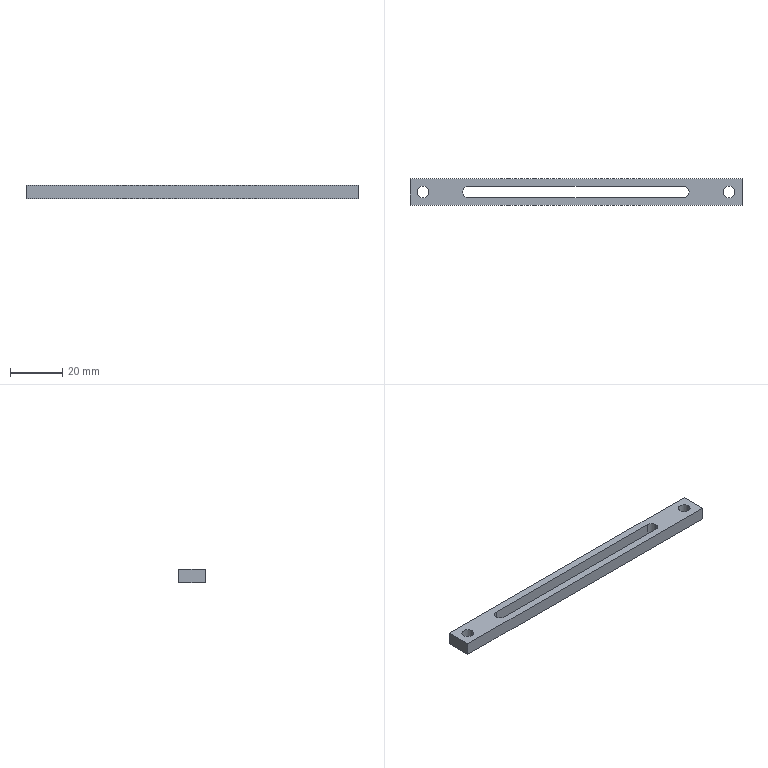Part | STEP file | 11-FG-B00311 | 1 solid | 15 faces | box 127 x 10 x 5 mm | volume 4266 mm3 | plane 8 | cylinder 7 | commonest cylinder face diameters 4.5 x7
STEP:
#1=CARTESIAN_POINT('',(106.75,5.,0.));
#2=VERTEX_POINT('',#1);
#3=CARTESIAN_POINT('',(104.5,7.25,0.));
#4=VERTEX_POINT('',#3);
#5=CARTESIAN_POINT('',(104.5,5.,0.));
#6=DIRECTION('',(0.,0.,1.));
#7=DIRECTION('',(1.,0.,0.));
#8=AXIS2_PLACEMENT_3D('',#5,#6,#7);
#9=CIRCLE('',#8,2.25);
#10=EDGE_CURVE('',#2,#4,#9,.T.);
#11=ORIENTED_EDGE('',*,*,#10,.F.);
#12=CARTESIAN_POINT('',(106.75,5.,5.));
#13=VERTEX_POINT('',#12);
#14=CARTESIAN_POINT('',(106.75,5.,0.));
#15=DIRECTION('',(0.,0.,1.));
#16=VECTOR('',#15,1000.);
#17=LINE('',#14,#16);
#18=EDGE_CURVE('',#2,#13,#17,.T.);
#19=ORIENTED_EDGE('',*,*,#18,.T.);
#20=CARTESIAN_POINT('',(104.5,7.25,5.));
#21=VERTEX_POINT('',#20);
#22=CARTESIAN_POINT('',(104.5,5.,5.));
#23=DIRECTION('',(0.,0.,1.));
#24=DIRECTION('',(1.,0.,0.));
#25=AXIS2_PLACEMENT_3D('',#22,#23,#24);
#26=CIRCLE('',#25,2.25);
#27=EDGE_CURVE('',#13,#21,#26,.T.);
#28=ORIENTED_EDGE('',*,*,#27,.T.);
#29=CARTESIAN_POINT('',(104.5,7.25,0.));
#30=DIRECTION('',(0.,0.,1.));
#31=VECTOR('',#30,1000.);
#32=LINE('',#29,#31);
#33=EDGE_CURVE('',#4,#21,#32,.T.);
#34=ORIENTED_EDGE('',*,*,#33,.F.);
#35=EDGE_LOOP('',(#11,#19,#28,#34));
#36=FACE_OUTER_BOUND('',#35,.T.);
#37=CARTESIAN_POINT('',(104.5,5.,0.));
#38=DIRECTION('',(0.,0.,1.));
#39=DIRECTION('',(1.,0.,0.));
#40=AXIS2_PLACEMENT_3D('',#37,#38,#39);
#41=CYLINDRICAL_SURFACE('',#40,2.25);
#42=ADVANCED_FACE('',(#36),#41,.F.);
#43=CARTESIAN_POINT('',(119.75,5.,0.));
#44=VERTEX_POINT('',#43);
#45=CARTESIAN_POINT('',(124.25,5.,0.));
#46=VERTEX_POINT('',#45);
#47=CARTESIAN_POINT('',(122.,5.,0.));
#48=DIRECTION('',(0.,0.,1.));
#49=DIRECTION('',(1.,0.,0.));
#50=AXIS2_PLACEMENT_3D('',#47,#48,#49);
#51=CIRCLE('',#50,2.25);
#52=EDGE_CURVE('',#44,#46,#51,.T.);
#53=ORIENTED_EDGE('',*,*,#52,.F.);
#54=CARTESIAN_POINT('',(119.75,5.,5.));
#55=VERTEX_POINT('',#54);
#56=CARTESIAN_POINT('',(119.75,5.,0.));
#57=DIRECTION('',(0.,0.,1.));
#58=VECTOR('',#57,1000.);
#59=LINE('',#56,#58);
#60=EDGE_CURVE('',#44,#55,#59,.T.);
#61=ORIENTED_EDGE('',*,*,#60,.T.);
#62=CARTESIAN_POINT('',(124.25,5.,5.));
#63=VERTEX_POINT('',#62);
#64=CARTESIAN_POINT('',(122.,5.,5.));
#65=DIRECTION('',(0.,0.,1.));
#66=DIRECTION('',(1.,0.,0.));
#67=AXIS2_PLACEMENT_3D('',#64,#65,#66);
#68=CIRCLE('',#67,2.25);
#69=EDGE_CURVE('',#55,#63,#68,.T.);
#70=ORIENTED_EDGE('',*,*,#69,.T.);
#71=CARTESIAN_POINT('',(124.25,5.,0.));
#72=DIRECTION('',(0.,0.,1.));
#73=VECTOR('',#72,1000.);
#74=LINE('',#71,#73);
#75=EDGE_CURVE('',#46,#63,#74,.T.);
#76=ORIENTED_EDGE('',*,*,#75,.F.);
#77=EDGE_LOOP('',(#53,#61,#70,#76));
#78=FACE_OUTER_BOUND('',#77,.T.);
#79=CARTESIAN_POINT('',(122.,5.,0.));
#80=DIRECTION('',(0.,0.,1.));
#81=DIRECTION('',(1.,0.,0.));
#82=AXIS2_PLACEMENT_3D('',#79,#80,#81);
#83=CYLINDRICAL_SURFACE('',#82,2.25);
#84=ADVANCED_FACE('',(#78),#83,.F.);
#85=CARTESIAN_POINT('',(2.75,5.,0.));
#86=VERTEX_POINT('',#85);
#87=CARTESIAN_POINT('',(7.25,5.,0.));
#88=VERTEX_POINT('',#87);
#89=CARTESIAN_POINT('',(5.,5.,0.));
#90=DIRECTION('',(0.,0.,1.));
#91=DIRECTION('',(1.,0.,0.));
#92=AXIS2_PLACEMENT_3D('',#89,#90,#91);
#93=CIRCLE('',#92,2.25);
#94=EDGE_CURVE('',#86,#88,#93,.T.);
#95=ORIENTED_EDGE('',*,*,#94,.F.);
#96=CARTESIAN_POINT('',(2.75,5.,5.));
#97=VERTEX_POINT('',#96);
#98=CARTESIAN_POINT('',(2.75,5.,0.));
#99=DIRECTION('',(0.,0.,1.));
#100=VECTOR('',#99,1000.);
#101=LINE('',#98,#100);
#102=EDGE_CURVE('',#86,#97,#101,.T.);
#103=ORIENTED_EDGE('',*,*,#102,.T.);
#104=CARTESIAN_POINT('',(7.25,5.,5.));
#105=VERTEX_POINT('',#104);
#106=CARTESIAN_POINT('',(5.,5.,5.));
#107=DIRECTION('',(0.,0.,1.));
#108=DIRECTION('',(1.,0.,0.));
#109=AXIS2_PLACEMENT_3D('',#106,#107,#108);
#110=CIRCLE('',#109,2.25);
#111=EDGE_CURVE('',#97,#105,#110,.T.);
#112=ORIENTED_EDGE('',*,*,#111,.T.);
#113=CARTESIAN_POINT('',(7.25,5.,0.));
#114=DIRECTION('',(0.,0.,1.));
#115=VECTOR('',#114,1000.);
#116=LINE('',#113,#115);
#117=EDGE_CURVE('',#88,#105,#116,.T.);
#118=ORIENTED_EDGE('',*,*,#117,.F.);
#119=EDGE_LOOP('',(#95,#103,#112,#118));
#120=FACE_OUTER_BOUND('',#119,.T.);
#121=CARTESIAN_POINT('',(5.,5.,0.));
#122=DIRECTION('',(0.,0.,1.));
#123=DIRECTION('',(1.,0.,0.));
#124=AXIS2_PLACEMENT_3D('',#121,#122,#123);
#125=CYLINDRICAL_SURFACE('',#124,2.25);
#126=ADVANCED_FACE('',(#120),#125,.F.);
#127=CARTESIAN_POINT('',(0.,10.,0.));
#128=VERTEX_POINT('',#127);
#129=CARTESIAN_POINT('',(0.,0.,0.));
#130=VERTEX_POINT('',#129);
#131=CARTESIAN_POINT('',(0.,0.,0.));
#132=DIRECTION('',(0.,-1.,0.));
#133=VECTOR('',#132,1000.);
#134=LINE('',#131,#133);
#135=EDGE_CURVE('',#128,#130,#134,.T.);
#136=ORIENTED_EDGE('',*,*,#135,.T.);
#137=CARTESIAN_POINT('',(0.,0.,5.));
#138=VERTEX_POINT('',#137);
#139=CARTESIAN_POINT('',(0.,0.,5.));
#140=DIRECTION('',(0.,0.,-1.));
#141=VECTOR('',#140,1000.);
#142=LINE('',#139,#141);
#143=EDGE_CURVE('',#138,#130,#142,.T.);
#144=ORIENTED_EDGE('',*,*,#143,.F.);
#145=CARTESIAN_POINT('',(0.,10.,5.));
#146=VERTEX_POINT('',#145);
#147=CARTESIAN_POINT('',(0.,0.,5.));
#148=DIRECTION('',(0.,-1.,0.));
#149=VECTOR('',#148,1000.);
#150=LINE('',#147,#149);
#151=EDGE_CURVE('',#146,#138,#150,.T.);
#152=ORIENTED_EDGE('',*,*,#151,.F.);
#153=CARTESIAN_POINT('',(0.,10.,5.));
#154=DIRECTION('',(0.,0.,-1.));
#155=VECTOR('',#154,1000.);
#156=LINE('',#153,#155);
#157=EDGE_CURVE('',#146,#128,#156,.T.);
#158=ORIENTED_EDGE('',*,*,#157,.T.);
#159=EDGE_LOOP('',(#136,#144,#152,#158));
#160=FACE_OUTER_BOUND('',#159,.T.);
#161=CARTESIAN_POINT('',(0.,0.,5.));
#162=DIRECTION('',(1.,0.,0.));
#163=DIRECTION('',(0.,0.,-1.));
#164=AXIS2_PLACEMENT_3D('',#161,#162,#163);
#165=PLANE('',#164);
#166=ADVANCED_FACE('',(#160),#165,.F.);
#167=CARTESIAN_POINT('',(127.,0.,0.));
#168=VERTEX_POINT('',#167);
#169=CARTESIAN_POINT('',(0.,0.,0.));
#170=DIRECTION('',(1.,0.,0.));
#171=VECTOR('',#170,1000.);
#172=LINE('',#169,#171);
#173=EDGE_CURVE('',#130,#168,#172,.T.);
#174=ORIENTED_EDGE('',*,*,#173,.T.);
#175=CARTESIAN_POINT('',(127.,0.,5.));
#176=VERTEX_POINT('',#175);
#177=CARTESIAN_POINT('',(127.,0.,5.));
#178=DIRECTION('',(0.,0.,-1.));
#179=VECTOR('',#178,1000.);
#180=LINE('',#177,#179);
#181=EDGE_CURVE('',#176,#168,#180,.T.);
#182=ORIENTED_EDGE('',*,*,#181,.F.);
#183=CARTESIAN_POINT('',(0.,0.,5.));
#184=DIRECTION('',(1.,0.,0.));
#185=VECTOR('',#184,1000.);
#186=LINE('',#183,#185);
#187=EDGE_CURVE('',#138,#176,#186,.T.);
#188=ORIENTED_EDGE('',*,*,#187,.F.);
#189=ORIENTED_EDGE('',*,*,#143,.T.);
#190=EDGE_LOOP('',(#174,#182,#188,#189));
#191=FACE_OUTER_BOUND('',#190,.T.);
#192=CARTESIAN_POINT('',(0.,0.,5.));
#193=DIRECTION('',(0.,1.,0.));
#194=DIRECTION('',(0.,0.,1.));
#195=AXIS2_PLACEMENT_3D('',#192,#193,#194);
#196=PLANE('',#195);
#197=ADVANCED_FACE('',(#191),#196,.F.);
#198=CARTESIAN_POINT('',(127.,10.,0.));
#199=VERTEX_POINT('',#198);
#200=CARTESIAN_POINT('',(127.,0.,0.));
#201=DIRECTION('',(0.,1.,0.));
#202=VECTOR('',#201,1000.);
#203=LINE('',#200,#202);
#204=EDGE_CURVE('',#168,#199,#203,.T.);
#205=ORIENTED_EDGE('',*,*,#204,.T.);
#206=CARTESIAN_POINT('',(127.,10.,5.));
#207=VERTEX_POINT('',#206);
#208=CARTESIAN_POINT('',(127.,10.,5.));
#209=DIRECTION('',(0.,0.,-1.));
#210=VECTOR('',#209,1000.);
#211=LINE('',#208,#210);
#212=EDGE_CURVE('',#207,#199,#211,.T.);
#213=ORIENTED_EDGE('',*,*,#212,.F.);
#214=CARTESIAN_POINT('',(127.,0.,5.));
#215=DIRECTION('',(0.,1.,0.));
#216=VECTOR('',#215,1000.);
#217=LINE('',#214,#216);
#218=EDGE_CURVE('',#176,#207,#217,.T.);
#219=ORIENTED_EDGE('',*,*,#218,.F.);
#220=ORIENTED_EDGE('',*,*,#181,.T.);
#221=EDGE_LOOP('',(#205,#213,#219,#220));
#222=FACE_OUTER_BOUND('',#221,.T.);
#223=CARTESIAN_POINT('',(127.,0.,5.));
#224=DIRECTION('',(-1.,0.,0.));
#225=DIRECTION('',(0.,0.,1.));
#226=AXIS2_PLACEMENT_3D('',#223,#224,#225);
#227=PLANE('',#226);
#228=ADVANCED_FACE('',(#222),#227,.F.);
#229=CARTESIAN_POINT('',(0.,10.,0.));
#230=DIRECTION('',(-1.,0.,0.));
#231=VECTOR('',#230,1000.);
#232=LINE('',#229,#231);
#233=EDGE_CURVE('',#199,#128,#232,.T.);
#234=ORIENTED_EDGE('',*,*,#233,.T.);
#235=ORIENTED_EDGE('',*,*,#157,.F.);
#236=CARTESIAN_POINT('',(0.,10.,5.));
#237=DIRECTION('',(-1.,0.,0.));
#238=VECTOR('',#237,1000.);
#239=LINE('',#236,#238);
#240=EDGE_CURVE('',#207,#146,#239,.T.);
#241=ORIENTED_EDGE('',*,*,#240,.F.);
#242=ORIENTED_EDGE('',*,*,#212,.T.);
#243=EDGE_LOOP('',(#234,#235,#241,#242));
#244=FACE_OUTER_BOUND('',#243,.T.);
#245=CARTESIAN_POINT('',(0.,10.,5.));
#246=DIRECTION('',(0.,-1.,0.));
#247=DIRECTION('',(0.,0.,-1.));
#248=AXIS2_PLACEMENT_3D('',#245,#246,#247);
#249=PLANE('',#248);
#250=ADVANCED_FACE('',(#244),#249,.F.);
#251=CARTESIAN_POINT('',(22.5,2.75,5.));
#252=VERTEX_POINT('',#251);
#253=CARTESIAN_POINT('',(104.5,2.75,5.));
#254=VERTEX_POINT('',#253);
#255=CARTESIAN_POINT('',(22.5,2.75,5.));
#256=DIRECTION('',(1.,0.,0.));
#257=VECTOR('',#256,1000.);
#258=LINE('',#255,#257);
#259=EDGE_CURVE('',#252,#254,#258,.T.);
#260=ORIENTED_EDGE('',*,*,#259,.F.);
#261=CARTESIAN_POINT('',(22.5,7.25,5.));
#262=VERTEX_POINT('',#261);
#263=CARTESIAN_POINT('',(22.5,5.,5.));
#264=DIRECTION('',(0.,0.,1.));
#265=DIRECTION('',(1.,0.,0.));
#266=AXIS2_PLACEMENT_3D('',#263,#264,#265);
#267=CIRCLE('',#266,2.25);
#268=EDGE_CURVE('',#262,#252,#267,.T.);
#269=ORIENTED_EDGE('',*,*,#268,.F.);
#270=CARTESIAN_POINT('',(22.5,7.25,5.));
#271=DIRECTION('',(-1.,0.,0.));
#272=VECTOR('',#271,1000.);
#273=LINE('',#270,#272);
#274=EDGE_CURVE('',#21,#262,#273,.T.);
#275=ORIENTED_EDGE('',*,*,#274,.F.);
#276=ORIENTED_EDGE('',*,*,#27,.F.);
#277=CARTESIAN_POINT('',(104.5,5.,5.));
#278=DIRECTION('',(0.,0.,1.));
#279=DIRECTION('',(1.,0.,0.));
#280=AXIS2_PLACEMENT_3D('',#277,#278,#279);
#281=CIRCLE('',#280,2.25);
#282=EDGE_CURVE('',#254,#13,#281,.T.);
#283=ORIENTED_EDGE('',*,*,#282,.F.);
#284=EDGE_LOOP('',(#260,#269,#275,#276,#283));
#285=FACE_BOUND('',#284,.T.);
#286=CARTESIAN_POINT('',(122.,5.,5.));
#287=DIRECTION('',(0.,0.,1.));
#288=DIRECTION('',(1.,0.,0.));
#289=AXIS2_PLACEMENT_3D('',#286,#287,#288);
#290=CIRCLE('',#289,2.25);
#291=EDGE_CURVE('',#63,#55,#290,.T.);
#292=ORIENTED_EDGE('',*,*,#291,.F.);
#293=ORIENTED_EDGE('',*,*,#69,.F.);
#294=EDGE_LOOP('',(#292,#293));
#295=FACE_BOUND('',#294,.T.);
#296=CARTESIAN_POINT('',(5.,5.,5.));
#297=DIRECTION('',(0.,0.,1.));
#298=DIRECTION('',(1.,0.,0.));
#299=AXIS2_PLACEMENT_3D('',#296,#297,#298);
#300=CIRCLE('',#299,2.25);
#301=EDGE_CURVE('',#105,#97,#300,.T.);
#302=ORIENTED_EDGE('',*,*,#301,.F.);
#303=ORIENTED_EDGE('',*,*,#111,.F.);
#304=EDGE_LOOP('',(#302,#303));
#305=FACE_BOUND('',#304,.T.);
#306=ORIENTED_EDGE('',*,*,#151,.T.);
#307=ORIENTED_EDGE('',*,*,#187,.T.);
#308=ORIENTED_EDGE('',*,*,#218,.T.);
#309=ORIENTED_EDGE('',*,*,#240,.T.);
#310=EDGE_LOOP('',(#306,#307,#308,#309));
#311=FACE_OUTER_BOUND('',#310,.T.);
#312=CARTESIAN_POINT('',(0.,10.,5.));
#313=DIRECTION('',(0.,0.,-1.));
#314=DIRECTION('',(-1.,0.,0.));
#315=AXIS2_PLACEMENT_3D('',#312,#313,#314);
#316=PLANE('',#315);
#317=ADVANCED_FACE('',(#285,#295,#305,#311),#316,.F.);
#318=CARTESIAN_POINT('',(22.5,7.25,0.));
#319=VERTEX_POINT('',#318);
#320=CARTESIAN_POINT('',(22.5,2.75,0.));
#321=VERTEX_POINT('',#320);
#322=CARTESIAN_POINT('',(22.5,5.,0.));
#323=DIRECTION('',(0.,0.,1.));
#324=DIRECTION('',(1.,0.,0.));
#325=AXIS2_PLACEMENT_3D('',#322,#323,#324);
#326=CIRCLE('',#325,2.25);
#327=EDGE_CURVE('',#319,#321,#326,.T.);
#328=ORIENTED_EDGE('',*,*,#327,.T.);
#329=CARTESIAN_POINT('',(104.5,2.75,0.));
#330=VERTEX_POINT('',#329);
#331=CARTESIAN_POINT('',(22.5,2.75,0.));
#332=DIRECTION('',(1.,0.,0.));
#333=VECTOR('',#332,1000.);
#334=LINE('',#331,#333);
#335=EDGE_CURVE('',#321,#330,#334,.T.);
#336=ORIENTED_EDGE('',*,*,#335,.T.);
#337=CARTESIAN_POINT('',(104.5,5.,0.));
#338=DIRECTION('',(0.,0.,1.));
#339=DIRECTION('',(1.,0.,0.));
#340=AXIS2_PLACEMENT_3D('',#337,#338,#339);
#341=CIRCLE('',#340,2.25);
#342=EDGE_CURVE('',#330,#2,#341,.T.);
#343=ORIENTED_EDGE('',*,*,#342,.T.);
#344=ORIENTED_EDGE('',*,*,#10,.T.);
#345=CARTESIAN_POINT('',(22.5,7.25,0.));
#346=DIRECTION('',(-1.,0.,0.));
#347=VECTOR('',#346,1000.);
#348=LINE('',#345,#347);
#349=EDGE_CURVE('',#4,#319,#348,.T.);
#350=ORIENTED_EDGE('',*,*,#349,.T.);
#351=EDGE_LOOP('',(#328,#336,#343,#344,#350));
#352=FACE_BOUND('',#351,.T.);
#353=CARTESIAN_POINT('',(122.,5.,0.));
#354=DIRECTION('',(0.,0.,1.));
#355=DIRECTION('',(1.,0.,0.));
#356=AXIS2_PLACEMENT_3D('',#353,#354,#355);
#357=CIRCLE('',#356,2.25);
#358=EDGE_CURVE('',#46,#44,#357,.T.);
#359=ORIENTED_EDGE('',*,*,#358,.T.);
#360=ORIENTED_EDGE('',*,*,#52,.T.);
#361=EDGE_LOOP('',(#359,#360));
#362=FACE_BOUND('',#361,.T.);
#363=CARTESIAN_POINT('',(5.,5.,0.));
#364=DIRECTION('',(0.,0.,1.));
#365=DIRECTION('',(1.,0.,0.));
#366=AXIS2_PLACEMENT_3D('',#363,#364,#365);
#367=CIRCLE('',#366,2.25);
#368=EDGE_CURVE('',#88,#86,#367,.T.);
#369=ORIENTED_EDGE('',*,*,#368,.T.);
#370=ORIENTED_EDGE('',*,*,#94,.T.);
#371=EDGE_LOOP('',(#369,#370));
#372=FACE_BOUND('',#371,.T.);
#373=ORIENTED_EDGE('',*,*,#135,.F.);
#374=ORIENTED_EDGE('',*,*,#233,.F.);
#375=ORIENTED_EDGE('',*,*,#204,.F.);
#376=ORIENTED_EDGE('',*,*,#173,.F.);
#377=EDGE_LOOP('',(#373,#374,#375,#376));
#378=FACE_OUTER_BOUND('',#377,.T.);
#379=CARTESIAN_POINT('',(0.,10.,0.));
#380=DIRECTION('',(0.,0.,-1.));
#381=DIRECTION('',(-1.,0.,0.));
#382=AXIS2_PLACEMENT_3D('',#379,#380,#381);
#383=PLANE('',#382);
#384=ADVANCED_FACE('',(#352,#362,#372,#378),#383,.T.);
#385=ORIENTED_EDGE('',*,*,#102,.F.);
#386=ORIENTED_EDGE('',*,*,#368,.F.);
#387=ORIENTED_EDGE('',*,*,#117,.T.);
#388=ORIENTED_EDGE('',*,*,#301,.T.);
#389=EDGE_LOOP('',(#385,#386,#387,#388));
#390=FACE_OUTER_BOUND('',#389,.T.);
#391=CARTESIAN_POINT('',(5.,5.,0.));
#392=DIRECTION('',(0.,0.,1.));
#393=DIRECTION('',(1.,0.,0.));
#394=AXIS2_PLACEMENT_3D('',#391,#392,#393);
#395=CYLINDRICAL_SURFACE('',#394,2.25);
#396=ADVANCED_FACE('',(#390),#395,.F.);
#397=ORIENTED_EDGE('',*,*,#60,.F.);
#398=ORIENTED_EDGE('',*,*,#358,.F.);
#399=ORIENTED_EDGE('',*,*,#75,.T.);
#400=ORIENTED_EDGE('',*,*,#291,.T.);
#401=EDGE_LOOP('',(#397,#398,#399,#400));
#402=FACE_OUTER_BOUND('',#401,.T.);
#403=CARTESIAN_POINT('',(122.,5.,0.));
#404=DIRECTION('',(0.,0.,1.));
#405=DIRECTION('',(1.,0.,0.));
#406=AXIS2_PLACEMENT_3D('',#403,#404,#405);
#407=CYLINDRICAL_SURFACE('',#406,2.25);
#408=ADVANCED_FACE('',(#402),#407,.F.);
#409=ORIENTED_EDGE('',*,*,#268,.T.);
#410=CARTESIAN_POINT('',(22.5,2.75,0.));
#411=DIRECTION('',(0.,0.,1.));
#412=VECTOR('',#411,1000.);
#413=LINE('',#410,#412);
#414=EDGE_CURVE('',#321,#252,#413,.T.);
#415=ORIENTED_EDGE('',*,*,#414,.F.);
#416=ORIENTED_EDGE('',*,*,#327,.F.);
#417=CARTESIAN_POINT('',(22.5,7.25,0.));
#418=DIRECTION('',(0.,0.,1.));
#419=VECTOR('',#418,1000.);
#420=LINE('',#417,#419);
#421=EDGE_CURVE('',#319,#262,#420,.T.);
#422=ORIENTED_EDGE('',*,*,#421,.T.);
#423=EDGE_LOOP('',(#409,#415,#416,#422));
#424=FACE_OUTER_BOUND('',#423,.T.);
#425=CARTESIAN_POINT('',(22.5,5.,0.));
#426=DIRECTION('',(0.,0.,1.));
#427=DIRECTION('',(1.,0.,0.));
#428=AXIS2_PLACEMENT_3D('',#425,#426,#427);
#429=CYLINDRICAL_SURFACE('',#428,2.25);
#430=ADVANCED_FACE('',(#424),#429,.F.);
#431=ORIENTED_EDGE('',*,*,#274,.T.);
#432=ORIENTED_EDGE('',*,*,#421,.F.);
#433=ORIENTED_EDGE('',*,*,#349,.F.);
#434=ORIENTED_EDGE('',*,*,#33,.T.);
#435=EDGE_LOOP('',(#431,#432,#433,#434));
#436=FACE_OUTER_BOUND('',#435,.T.);
#437=CARTESIAN_POINT('',(22.5,7.25,0.));
#438=DIRECTION('',(0.,1.,0.));
#439=DIRECTION('',(-1.,0.,0.));
#440=AXIS2_PLACEMENT_3D('',#437,#438,#439);
#441=PLANE('',#440);
#442=ADVANCED_FACE('',(#436),#441,.F.);
#443=ORIENTED_EDGE('',*,*,#18,.F.);
#444=ORIENTED_EDGE('',*,*,#342,.F.);
#445=CARTESIAN_POINT('',(104.5,2.75,0.));
#446=DIRECTION('',(0.,0.,1.));
#447=VECTOR('',#446,1000.);
#448=LINE('',#445,#447);
#449=EDGE_CURVE('',#330,#254,#448,.T.);
#450=ORIENTED_EDGE('',*,*,#449,.T.);
#451=ORIENTED_EDGE('',*,*,#282,.T.);
#452=EDGE_LOOP('',(#443,#444,#450,#451));
#453=FACE_OUTER_BOUND('',#452,.T.);
#454=CARTESIAN_POINT('',(104.5,5.,0.));
#455=DIRECTION('',(0.,0.,1.));
#456=DIRECTION('',(1.,0.,0.));
#457=AXIS2_PLACEMENT_3D('',#454,#455,#456);
#458=CYLINDRICAL_SURFACE('',#457,2.25);
#459=ADVANCED_FACE('',(#453),#458,.F.);
#460=ORIENTED_EDGE('',*,*,#259,.T.);
#461=ORIENTED_EDGE('',*,*,#449,.F.);
#462=ORIENTED_EDGE('',*,*,#335,.F.);
#463=ORIENTED_EDGE('',*,*,#414,.T.);
#464=EDGE_LOOP('',(#460,#461,#462,#463));
#465=FACE_OUTER_BOUND('',#464,.T.);
#466=CARTESIAN_POINT('',(22.5,2.75,0.));
#467=DIRECTION('',(0.,-1.,0.));
#468=DIRECTION('',(1.,0.,0.));
#469=AXIS2_PLACEMENT_3D('',#466,#467,#468);
#470=PLANE('',#469);
#471=ADVANCED_FACE('',(#465),#470,.F.);
#472=CLOSED_SHELL('',(#42,#84,#126,#166,#197,#228,#250,#317,#384,#396,#408,#430,#442,#459,#471));
#473=MANIFOLD_SOLID_BREP('',#472);
#474=CARTESIAN_POINT('',(0.,0.,0.));
#475=DIRECTION('',(0.,0.,1.));
#476=DIRECTION('',(1.,0.,0.));
#477=AXIS2_PLACEMENT_3D('',#474,#475,#476);
#478=(LENGTH_UNIT()NAMED_UNIT(*)SI_UNIT(.MILLI.,.METRE.));
#479=UNCERTAINTY_MEASURE_WITH_UNIT(LENGTH_MEASURE(0.00001),#478,'','');
#480=(NAMED_UNIT(*)PLANE_ANGLE_UNIT()SI_UNIT($,.RADIAN.));
#481=(NAMED_UNIT(*)SI_UNIT($,.STERADIAN.)SOLID_ANGLE_UNIT());
#482=(GEOMETRIC_REPRESENTATION_CONTEXT(3)GLOBAL_UNCERTAINTY_ASSIGNED_CONTEXT((#479))GLOBAL_UNIT_ASSIGNED_CONTEXT((#478,#480,#481))REPRESENTATION_CONTEXT('',''));
#483=ADVANCED_BREP_SHAPE_REPRESENTATION('',(#473,#477),#482);